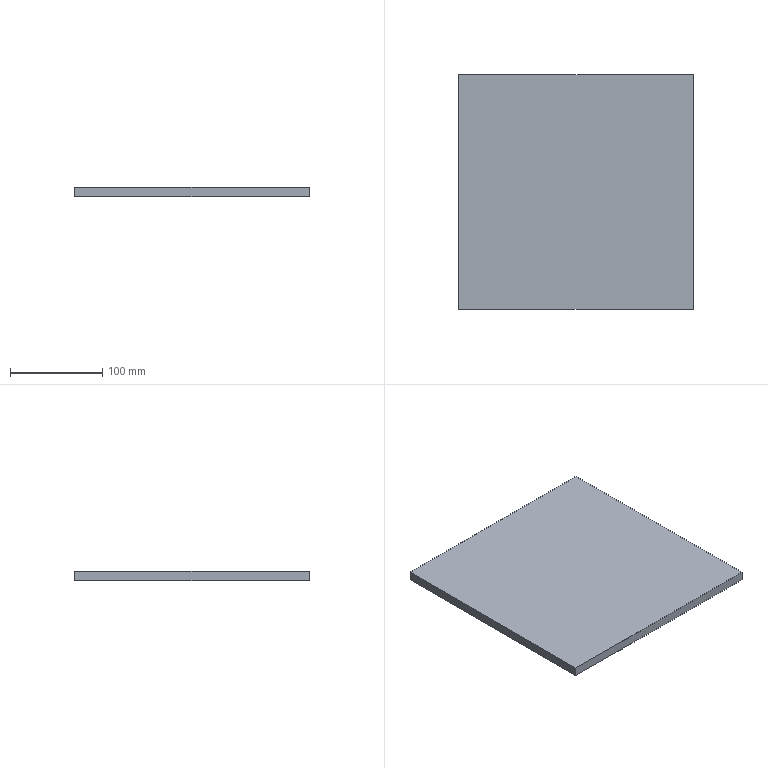Part | SolidWorks | features Extrusion 1 | 1 solid | 6 faces | box 254 x 254 x 10 mm | volume 645160 mm3 | plane 6
STEP:
#1=CARTESIAN_POINT('',(-127.,127.,-5.));
#2=VERTEX_POINT('',#1);
#3=CARTESIAN_POINT('',(-127.,-127.,-5.));
#4=VERTEX_POINT('',#3);
#5=CARTESIAN_POINT('',(-127.,127.,-5.));
#6=DIRECTION('',(0.,-1.,0.));
#7=VECTOR('',#6,1000.);
#8=LINE('',#5,#7);
#9=EDGE_CURVE('',#2,#4,#8,.T.);
#10=ORIENTED_EDGE('',*,*,#9,.T.);
#11=CARTESIAN_POINT('',(-127.,-127.,5.));
#12=VERTEX_POINT('',#11);
#13=CARTESIAN_POINT('',(-127.,-127.,5.));
#14=DIRECTION('',(0.,0.,-1.));
#15=VECTOR('',#14,1000.);
#16=LINE('',#13,#15);
#17=EDGE_CURVE('',#12,#4,#16,.T.);
#18=ORIENTED_EDGE('',*,*,#17,.F.);
#19=CARTESIAN_POINT('',(-127.,127.,5.));
#20=VERTEX_POINT('',#19);
#21=CARTESIAN_POINT('',(-127.,127.,5.));
#22=DIRECTION('',(0.,-1.,0.));
#23=VECTOR('',#22,1000.);
#24=LINE('',#21,#23);
#25=EDGE_CURVE('',#20,#12,#24,.T.);
#26=ORIENTED_EDGE('',*,*,#25,.F.);
#27=CARTESIAN_POINT('',(-127.,127.,5.));
#28=DIRECTION('',(0.,0.,-1.));
#29=VECTOR('',#28,1000.);
#30=LINE('',#27,#29);
#31=EDGE_CURVE('',#20,#2,#30,.T.);
#32=ORIENTED_EDGE('',*,*,#31,.T.);
#33=EDGE_LOOP('',(#10,#18,#26,#32));
#34=FACE_OUTER_BOUND('',#33,.T.);
#35=CARTESIAN_POINT('',(-127.,127.,5.));
#36=DIRECTION('',(1.,0.,0.));
#37=DIRECTION('',(0.,1.,0.));
#38=AXIS2_PLACEMENT_3D('',#35,#36,#37);
#39=PLANE('',#38);
#40=ADVANCED_FACE('',(#34),#39,.F.);
#41=CARTESIAN_POINT('',(127.,-127.,-5.));
#42=VERTEX_POINT('',#41);
#43=CARTESIAN_POINT('',(-127.,-127.,-5.));
#44=DIRECTION('',(1.,0.,0.));
#45=VECTOR('',#44,1000.);
#46=LINE('',#43,#45);
#47=EDGE_CURVE('',#4,#42,#46,.T.);
#48=ORIENTED_EDGE('',*,*,#47,.T.);
#49=CARTESIAN_POINT('',(127.,-127.,5.));
#50=VERTEX_POINT('',#49);
#51=CARTESIAN_POINT('',(127.,-127.,5.));
#52=DIRECTION('',(0.,0.,-1.));
#53=VECTOR('',#52,1000.);
#54=LINE('',#51,#53);
#55=EDGE_CURVE('',#50,#42,#54,.T.);
#56=ORIENTED_EDGE('',*,*,#55,.F.);
#57=CARTESIAN_POINT('',(-127.,-127.,5.));
#58=DIRECTION('',(1.,0.,0.));
#59=VECTOR('',#58,1000.);
#60=LINE('',#57,#59);
#61=EDGE_CURVE('',#12,#50,#60,.T.);
#62=ORIENTED_EDGE('',*,*,#61,.F.);
#63=ORIENTED_EDGE('',*,*,#17,.T.);
#64=EDGE_LOOP('',(#48,#56,#62,#63));
#65=FACE_OUTER_BOUND('',#64,.T.);
#66=CARTESIAN_POINT('',(-127.,-127.,5.));
#67=DIRECTION('',(0.,1.,0.));
#68=DIRECTION('',(0.,0.,1.));
#69=AXIS2_PLACEMENT_3D('',#66,#67,#68);
#70=PLANE('',#69);
#71=ADVANCED_FACE('',(#65),#70,.F.);
#72=CARTESIAN_POINT('',(127.,127.,-5.));
#73=VERTEX_POINT('',#72);
#74=CARTESIAN_POINT('',(127.,127.,-5.));
#75=DIRECTION('',(0.,1.,0.));
#76=VECTOR('',#75,1000.);
#77=LINE('',#74,#76);
#78=EDGE_CURVE('',#42,#73,#77,.T.);
#79=ORIENTED_EDGE('',*,*,#78,.T.);
#80=CARTESIAN_POINT('',(127.,127.,5.));
#81=VERTEX_POINT('',#80);
#82=CARTESIAN_POINT('',(127.,127.,5.));
#83=DIRECTION('',(0.,0.,-1.));
#84=VECTOR('',#83,1000.);
#85=LINE('',#82,#84);
#86=EDGE_CURVE('',#81,#73,#85,.T.);
#87=ORIENTED_EDGE('',*,*,#86,.F.);
#88=CARTESIAN_POINT('',(127.,127.,5.));
#89=DIRECTION('',(0.,1.,0.));
#90=VECTOR('',#89,1000.);
#91=LINE('',#88,#90);
#92=EDGE_CURVE('',#50,#81,#91,.T.);
#93=ORIENTED_EDGE('',*,*,#92,.F.);
#94=ORIENTED_EDGE('',*,*,#55,.T.);
#95=EDGE_LOOP('',(#79,#87,#93,#94));
#96=FACE_OUTER_BOUND('',#95,.T.);
#97=CARTESIAN_POINT('',(127.,127.,5.));
#98=DIRECTION('',(-1.,0.,0.));
#99=DIRECTION('',(0.,-1.,0.));
#100=AXIS2_PLACEMENT_3D('',#97,#98,#99);
#101=PLANE('',#100);
#102=ADVANCED_FACE('',(#96),#101,.F.);
#103=CARTESIAN_POINT('',(-127.,127.,-5.));
#104=DIRECTION('',(-1.,0.,0.));
#105=VECTOR('',#104,1000.);
#106=LINE('',#103,#105);
#107=EDGE_CURVE('',#73,#2,#106,.T.);
#108=ORIENTED_EDGE('',*,*,#107,.T.);
#109=ORIENTED_EDGE('',*,*,#31,.F.);
#110=CARTESIAN_POINT('',(-127.,127.,5.));
#111=DIRECTION('',(-1.,0.,0.));
#112=VECTOR('',#111,1000.);
#113=LINE('',#110,#112);
#114=EDGE_CURVE('',#81,#20,#113,.T.);
#115=ORIENTED_EDGE('',*,*,#114,.F.);
#116=ORIENTED_EDGE('',*,*,#86,.T.);
#117=EDGE_LOOP('',(#108,#109,#115,#116));
#118=FACE_OUTER_BOUND('',#117,.T.);
#119=CARTESIAN_POINT('',(-127.,127.,5.));
#120=DIRECTION('',(0.,-1.,0.));
#121=DIRECTION('',(0.,0.,-1.));
#122=AXIS2_PLACEMENT_3D('',#119,#120,#121);
#123=PLANE('',#122);
#124=ADVANCED_FACE('',(#118),#123,.F.);
#125=ORIENTED_EDGE('',*,*,#25,.T.);
#126=ORIENTED_EDGE('',*,*,#61,.T.);
#127=ORIENTED_EDGE('',*,*,#92,.T.);
#128=ORIENTED_EDGE('',*,*,#114,.T.);
#129=EDGE_LOOP('',(#125,#126,#127,#128));
#130=FACE_OUTER_BOUND('',#129,.T.);
#131=CARTESIAN_POINT('',(0.,0.,5.));
#132=DIRECTION('',(0.,0.,1.));
#133=DIRECTION('',(1.,0.,0.));
#134=AXIS2_PLACEMENT_3D('',#131,#132,#133);
#135=PLANE('',#134);
#136=ADVANCED_FACE('',(#130),#135,.T.);
#137=ORIENTED_EDGE('',*,*,#9,.F.);
#138=ORIENTED_EDGE('',*,*,#107,.F.);
#139=ORIENTED_EDGE('',*,*,#78,.F.);
#140=ORIENTED_EDGE('',*,*,#47,.F.);
#141=EDGE_LOOP('',(#137,#138,#139,#140));
#142=FACE_OUTER_BOUND('',#141,.T.);
#143=CARTESIAN_POINT('',(0.,0.,-5.));
#144=DIRECTION('',(0.,0.,1.));
#145=DIRECTION('',(1.,0.,0.));
#146=AXIS2_PLACEMENT_3D('',#143,#144,#145);
#147=PLANE('',#146);
#148=ADVANCED_FACE('',(#142),#147,.F.);
#149=CLOSED_SHELL('',(#40,#71,#102,#124,#136,#148));
#150=MANIFOLD_SOLID_BREP('',#149);
#151=CARTESIAN_POINT('',(0.,0.,0.));
#152=DIRECTION('',(0.,0.,1.));
#153=DIRECTION('',(1.,0.,0.));
#154=AXIS2_PLACEMENT_3D('',#151,#152,#153);
#155=(LENGTH_UNIT()NAMED_UNIT(*)SI_UNIT(.MILLI.,.METRE.));
#156=UNCERTAINTY_MEASURE_WITH_UNIT(LENGTH_MEASURE(0.00001),#155,'','');
#157=(NAMED_UNIT(*)PLANE_ANGLE_UNIT()SI_UNIT($,.RADIAN.));
#158=(NAMED_UNIT(*)SI_UNIT($,.STERADIAN.)SOLID_ANGLE_UNIT());
#159=(GEOMETRIC_REPRESENTATION_CONTEXT(3)GLOBAL_UNCERTAINTY_ASSIGNED_CONTEXT((#156))GLOBAL_UNIT_ASSIGNED_CONTEXT((#155,#157,#158))REPRESENTATION_CONTEXT('',''));
#160=ADVANCED_BREP_SHAPE_REPRESENTATION('',(#150,#154),#159);